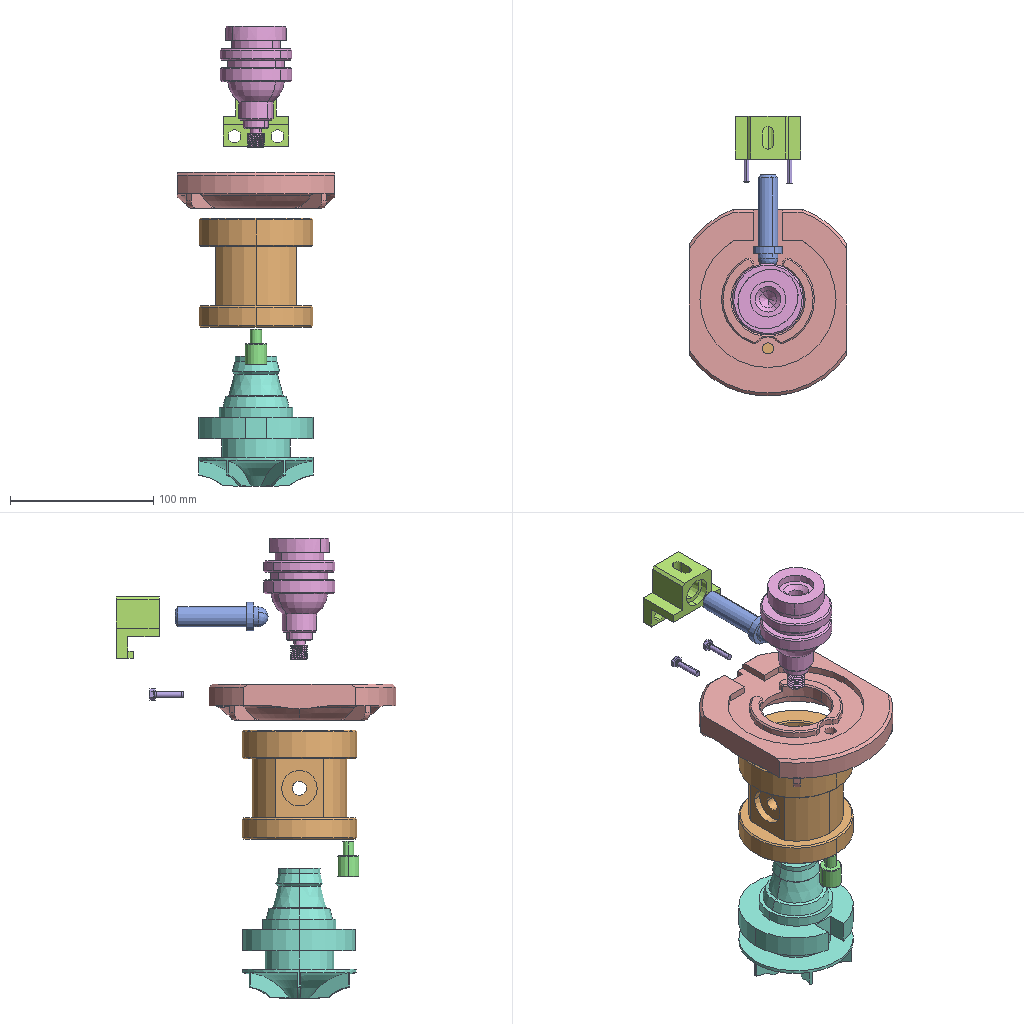Assembly | SolidWorks | 8 different items | 9 placed | box 110 x 195 x 321 mm
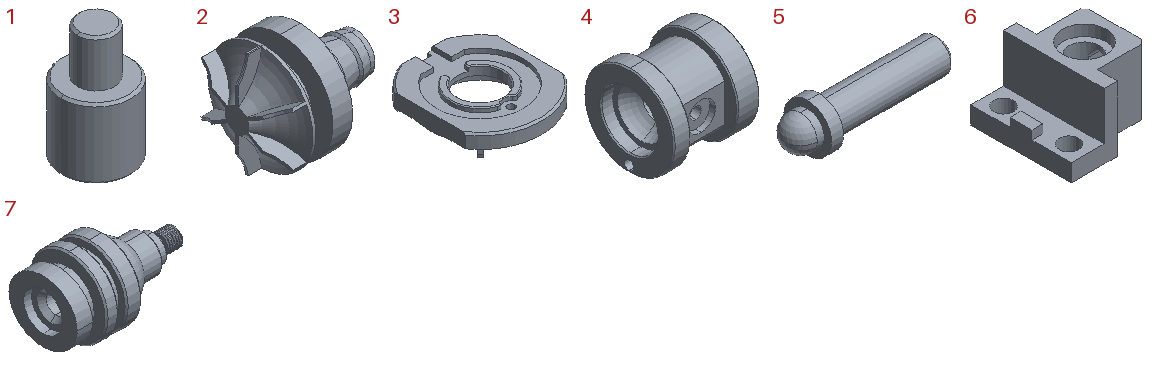Parts list (item | name | quantity | size | volume | features):
1 | - | x2 | 15 x 15 x 25 mm | 3139 mm3 | features Chamfer 1, Extrusion 1, ICE 1
2 | - | x1 | 90.5 x 80 x 80 mm | 181768 mm3 | features ICE 2, HoleWzd 1, RevCut 1, Revolution 1
3 | - | x1 | 110 x 130.5 x 25 mm | 159387 mm3 | features ICE 8, Chamfer 2, Fillet 2, Extrusion 1, HoleWzd 1, Revolution 1
4 | - | x1 | 76.2 x 80 x 80 mm | 211885 mm3 | features ICE 5, Chamfer 1, MirrorPattern 1, Revolution 1
5 | - | x1 | 65 x 20 x 20 mm | 10368 mm3 | features Revolution 1
6 | - | x1 | 43 x 46 x 30 mm | 25082 mm3 | features ICE 4, Chamfer 1, Extrusion 1
7 | - | x1 | 84.7 x 50 x 50 mm | 76525 mm3 | features Chamfer 1, Helix 1, ICE 1, RevCut 1, Revolution 1, SweepCut 1
8 | cross recessed hex bolts indentation gb | x1 | - | - | -
Mates (type | each side: item.copy, entity, surface, feature):
Concentric | 5.1 face cylinder Revolve1 | 6.1 face cylinder Boss-Extrude1
Coincident | 3.1 face plane Boss-Extrude1 | 6.1 face plane Cut-Extrude1
Coincident | 3.1 face plane Cut-Extrude3 | 6.1 face plane Boss-Extrude2
Concentric | 3.1 face cylinder M8 Tapped Hole1 | 6.1 face cylinder Boss-Extrude1
Concentric | 3.1 face cylinder Cut-Extrude6 | 4.1 face cylinder Revolve1
Concentric | 3.1 face cylinder Cut-Extrude4 | 4.1 face cylinder Cut-Extrude5
Coincident | 3.1 face plane Cut-Extrude6 | 4.1 face plane Revolve1
Concentric | 2.1 face cylinder Revolve1 | 4.1 face cylinder Revolve1
Concentric | 4.1 face cylinder Cut-Extrude4 | 1.1 face cylinder Boss-Extrude2
Coincident | 4.1 face plane Revolve1 | 1.1 face plane Boss-Extrude1
Tangent | 1.1 face cylinder Boss-Extrude1 | 2.1 face plane Cut-Extrude1
Tangent | 2.1 face plane Cut-Extrude1 | 1.1 face cylinder Boss-Extrude1
DistanceDim | 2.1 face plane Revolve1 | 4.1 face plane Revolve1
Concentric | 7.1 face cylinder Revolve1 | 4.1 face cylinder Revolve1
Coincident | 7.1 face plane Revolve1 | 2.1 face plane Revolve1